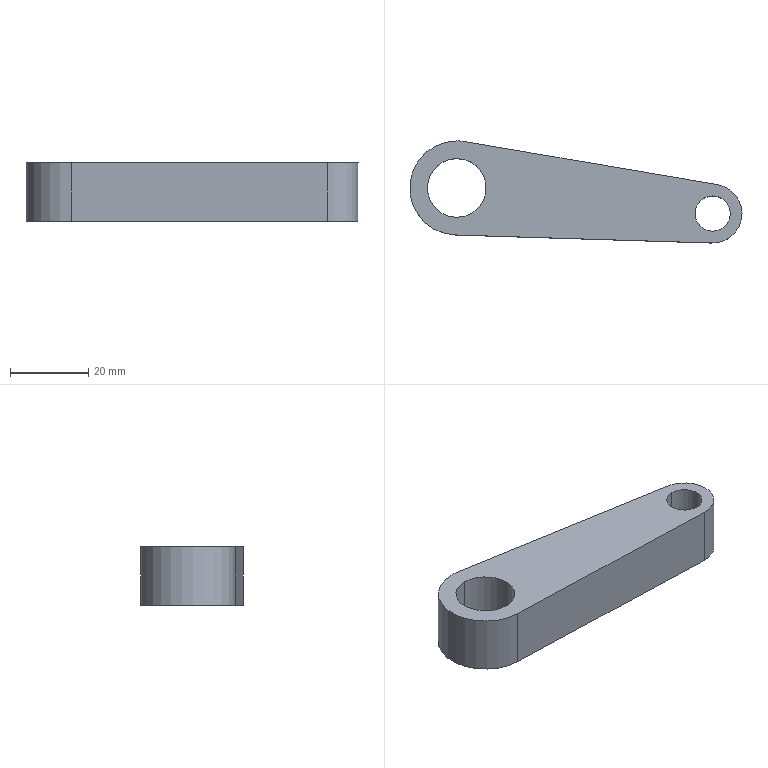Part | SolidWorks | features BaseBody 1 | 1 solid | 11 faces | box 84.765 x 26.042 x 15 mm | volume 20344 mm3 | cylinder 7 | plane 4 | commonest cylinder face diameters 15 x3 9 x2 24 x2
STEP:
#1=CARTESIAN_POINT('',(0.3749,23.994,15.));
#2=VERTEX_POINT('',#1);
#3=CARTESIAN_POINT('',(0.000000002,0.000000004,15.));
#4=VERTEX_POINT('',#3);
#5=CARTESIAN_POINT('',(0.3749,11.994,15.));
#6=DIRECTION('',(0.,0.,1.));
#7=DIRECTION('',(0.,1.,0.));
#8=AXIS2_PLACEMENT_3D('',#5,#6,#7);
#9=CIRCLE('',#8,12.);
#10=EDGE_CURVE('',#2,#4,#9,.T.);
#11=ORIENTED_EDGE('',*,*,#10,.F.);
#12=CARTESIAN_POINT('',(0.3749,23.994,0.));
#13=VERTEX_POINT('',#12);
#14=CARTESIAN_POINT('',(0.3749,23.994,15.));
#15=DIRECTION('',(0.,0.,-1.));
#16=VECTOR('',#15,1000.);
#17=LINE('',#14,#16);
#18=EDGE_CURVE('',#2,#13,#17,.T.);
#19=ORIENTED_EDGE('',*,*,#18,.T.);
#20=CARTESIAN_POINT('',(0.000000002,0.,0.));
#21=VERTEX_POINT('',#20);
#22=CARTESIAN_POINT('',(0.3749,11.994,0.));
#23=DIRECTION('',(0.,0.,-1.));
#24=DIRECTION('',(0.,1.,0.));
#25=AXIS2_PLACEMENT_3D('',#22,#23,#24);
#26=CIRCLE('',#25,12.);
#27=EDGE_CURVE('',#21,#13,#26,.T.);
#28=ORIENTED_EDGE('',*,*,#27,.F.);
#29=CARTESIAN_POINT('',(0.000000004,0.,7.5));
#30=DIRECTION('',(0.,0.,-1.));
#31=VECTOR('',#30,1000.);
#32=LINE('',#29,#31);
#33=EDGE_CURVE('',#4,#21,#32,.T.);
#34=ORIENTED_EDGE('',*,*,#33,.F.);
#35=EDGE_LOOP('',(#11,#19,#28,#34));
#36=FACE_OUTER_BOUND('',#35,.T.);
#37=CARTESIAN_POINT('',(0.3749,11.994,15.));
#38=DIRECTION('',(0.,0.,-1.));
#39=DIRECTION('',(0.,1.,0.));
#40=AXIS2_PLACEMENT_3D('',#37,#38,#39);
#41=CYLINDRICAL_SURFACE('',#40,12.);
#42=ADVANCED_FACE('',(#36),#41,.T.);
#43=CARTESIAN_POINT('',(65.64,0.9519,15.));
#44=VERTEX_POINT('',#43);
#45=CARTESIAN_POINT('',(65.64,9.952,15.));
#46=VERTEX_POINT('',#45);
#47=CARTESIAN_POINT('',(65.64,5.452,15.));
#48=DIRECTION('',(0.,0.,-1.));
#49=DIRECTION('',(0.,1.,0.));
#50=AXIS2_PLACEMENT_3D('',#47,#48,#49);
#51=CIRCLE('',#50,4.5);
#52=EDGE_CURVE('',#44,#46,#51,.T.);
#53=ORIENTED_EDGE('',*,*,#52,.F.);
#54=CARTESIAN_POINT('',(65.64,0.9519,0.));
#55=VERTEX_POINT('',#54);
#56=CARTESIAN_POINT('',(65.64,0.9519,15.));
#57=DIRECTION('',(0.,0.,-1.));
#58=VECTOR('',#57,1000.);
#59=LINE('',#56,#58);
#60=EDGE_CURVE('',#44,#55,#59,.T.);
#61=ORIENTED_EDGE('',*,*,#60,.T.);
#62=CARTESIAN_POINT('',(65.64,9.952,0.));
#63=VERTEX_POINT('',#62);
#64=CARTESIAN_POINT('',(65.64,5.452,0.));
#65=DIRECTION('',(0.,0.,-1.));
#66=DIRECTION('',(0.,1.,0.));
#67=AXIS2_PLACEMENT_3D('',#64,#65,#66);
#68=CIRCLE('',#67,4.5);
#69=EDGE_CURVE('',#55,#63,#68,.T.);
#70=ORIENTED_EDGE('',*,*,#69,.T.);
#71=CARTESIAN_POINT('',(65.64,9.952,15.));
#72=DIRECTION('',(0.,0.,-1.));
#73=VECTOR('',#72,1000.);
#74=LINE('',#71,#73);
#75=EDGE_CURVE('',#46,#63,#74,.T.);
#76=ORIENTED_EDGE('',*,*,#75,.F.);
#77=EDGE_LOOP('',(#53,#61,#70,#76));
#78=FACE_OUTER_BOUND('',#77,.T.);
#79=CARTESIAN_POINT('',(65.64,5.452,15.));
#80=DIRECTION('',(0.,0.,-1.));
#81=DIRECTION('',(0.,1.,0.));
#82=AXIS2_PLACEMENT_3D('',#79,#80,#81);
#83=CYLINDRICAL_SURFACE('',#82,4.5);
#84=ADVANCED_FACE('',(#78),#83,.F.);
#85=CARTESIAN_POINT('',(0.3749,4.494,15.));
#86=VERTEX_POINT('',#85);
#87=CARTESIAN_POINT('',(0.3749,19.494,15.));
#88=VERTEX_POINT('',#87);
#89=CARTESIAN_POINT('',(0.3749,11.994,15.));
#90=DIRECTION('',(0.,0.,-1.));
#91=DIRECTION('',(0.,1.,0.));
#92=AXIS2_PLACEMENT_3D('',#89,#90,#91);
#93=CIRCLE('',#92,7.5);
#94=EDGE_CURVE('',#86,#88,#93,.T.);
#95=ORIENTED_EDGE('',*,*,#94,.F.);
#96=CARTESIAN_POINT('',(0.3749,4.494,0.));
#97=VERTEX_POINT('',#96);
#98=CARTESIAN_POINT('',(0.3749,4.494,15.));
#99=DIRECTION('',(0.,0.,-1.));
#100=VECTOR('',#99,1000.);
#101=LINE('',#98,#100);
#102=EDGE_CURVE('',#86,#97,#101,.T.);
#103=ORIENTED_EDGE('',*,*,#102,.T.);
#104=CARTESIAN_POINT('',(0.3749,19.494,0.));
#105=VERTEX_POINT('',#104);
#106=CARTESIAN_POINT('',(0.3749,11.994,0.));
#107=DIRECTION('',(0.,0.,-1.));
#108=DIRECTION('',(0.,1.,0.));
#109=AXIS2_PLACEMENT_3D('',#106,#107,#108);
#110=CIRCLE('',#109,7.5);
#111=EDGE_CURVE('',#97,#105,#110,.T.);
#112=ORIENTED_EDGE('',*,*,#111,.T.);
#113=CARTESIAN_POINT('',(0.3749,19.494,15.));
#114=DIRECTION('',(0.,0.,-1.));
#115=VECTOR('',#114,1000.);
#116=LINE('',#113,#115);
#117=EDGE_CURVE('',#88,#105,#116,.T.);
#118=ORIENTED_EDGE('',*,*,#117,.F.);
#119=EDGE_LOOP('',(#95,#103,#112,#118));
#120=FACE_OUTER_BOUND('',#119,.T.);
#121=CARTESIAN_POINT('',(0.3749,11.994,15.));
#122=DIRECTION('',(0.,0.,-1.));
#123=DIRECTION('',(0.,1.,0.));
#124=AXIS2_PLACEMENT_3D('',#121,#122,#123);
#125=CYLINDRICAL_SURFACE('',#124,7.5);
#126=ADVANCED_FACE('',(#120),#125,.F.);
#127=ORIENTED_EDGE('',*,*,#18,.F.);
#128=CARTESIAN_POINT('',(2.388,23.824,15.));
#129=VERTEX_POINT('',#128);
#130=CARTESIAN_POINT('',(0.3749,11.994,15.));
#131=DIRECTION('',(0.,0.,1.));
#132=DIRECTION('',(0.,1.,0.));
#133=AXIS2_PLACEMENT_3D('',#130,#131,#132);
#134=CIRCLE('',#133,12.);
#135=EDGE_CURVE('',#129,#2,#134,.T.);
#136=ORIENTED_EDGE('',*,*,#135,.F.);
#137=CARTESIAN_POINT('',(2.388,23.824,0.));
#138=VERTEX_POINT('',#137);
#139=CARTESIAN_POINT('',(2.388,23.824,7.5));
#140=DIRECTION('',(0.,0.,1.));
#141=VECTOR('',#140,1000.);
#142=LINE('',#139,#141);
#143=EDGE_CURVE('',#138,#129,#142,.T.);
#144=ORIENTED_EDGE('',*,*,#143,.F.);
#145=CARTESIAN_POINT('',(0.3749,11.994,0.));
#146=DIRECTION('',(0.,0.,-1.));
#147=DIRECTION('',(0.,1.,0.));
#148=AXIS2_PLACEMENT_3D('',#145,#146,#147);
#149=CIRCLE('',#148,12.);
#150=EDGE_CURVE('',#13,#138,#149,.T.);
#151=ORIENTED_EDGE('',*,*,#150,.F.);
#152=EDGE_LOOP('',(#127,#136,#144,#151));
#153=FACE_OUTER_BOUND('',#152,.T.);
#154=CARTESIAN_POINT('',(0.3749,11.994,15.));
#155=DIRECTION('',(0.,0.,-1.));
#156=DIRECTION('',(0.,1.,0.));
#157=AXIS2_PLACEMENT_3D('',#154,#155,#156);
#158=CYLINDRICAL_SURFACE('',#157,12.);
#159=ADVANCED_FACE('',(#153),#158,.T.);
#160=CARTESIAN_POINT('',(65.64,5.452,15.));
#161=DIRECTION('',(0.,0.,-1.));
#162=DIRECTION('',(0.,1.,0.));
#163=AXIS2_PLACEMENT_3D('',#160,#161,#162);
#164=CIRCLE('',#163,4.5);
#165=EDGE_CURVE('',#46,#44,#164,.T.);
#166=ORIENTED_EDGE('',*,*,#165,.T.);
#167=ORIENTED_EDGE('',*,*,#52,.T.);
#168=EDGE_LOOP('',(#166,#167));
#169=FACE_BOUND('',#168,.T.);
#170=CARTESIAN_POINT('',(0.3749,11.994,15.));
#171=DIRECTION('',(0.,0.,-1.));
#172=DIRECTION('',(0.,1.,0.));
#173=AXIS2_PLACEMENT_3D('',#170,#171,#172);
#174=CIRCLE('',#173,7.5);
#175=EDGE_CURVE('',#88,#86,#174,.T.);
#176=ORIENTED_EDGE('',*,*,#175,.T.);
#177=ORIENTED_EDGE('',*,*,#94,.T.);
#178=EDGE_LOOP('',(#176,#177));
#179=FACE_BOUND('',#178,.T.);
#180=CARTESIAN_POINT('',(66.898,12.846,15.));
#181=VERTEX_POINT('',#180);
#182=CARTESIAN_POINT('',(66.898,12.846,15.));
#183=DIRECTION('',(-0.9858,0.1678,0.));
#184=VECTOR('',#183,1000.);
#185=LINE('',#182,#184);
#186=EDGE_CURVE('',#181,#129,#185,.T.);
#187=ORIENTED_EDGE('',*,*,#186,.T.);
#188=ORIENTED_EDGE('',*,*,#135,.T.);
#189=ORIENTED_EDGE('',*,*,#10,.T.);
#190=CARTESIAN_POINT('',(65.406,-2.044,15.));
#191=VERTEX_POINT('',#190);
#192=CARTESIAN_POINT('',(0.000000015,0.000000009,15.));
#193=DIRECTION('',(0.9995,-0.03124,0.));
#194=VECTOR('',#193,1000.);
#195=LINE('',#192,#194);
#196=EDGE_CURVE('',#4,#191,#195,.T.);
#197=ORIENTED_EDGE('',*,*,#196,.T.);
#198=CARTESIAN_POINT('',(65.64,5.452,15.));
#199=DIRECTION('',(0.,0.,1.));
#200=DIRECTION('',(0.,1.,0.));
#201=AXIS2_PLACEMENT_3D('',#198,#199,#200);
#202=CIRCLE('',#201,7.5);
#203=EDGE_CURVE('',#191,#181,#202,.T.);
#204=ORIENTED_EDGE('',*,*,#203,.T.);
#205=EDGE_LOOP('',(#187,#188,#189,#197,#204));
#206=FACE_OUTER_BOUND('',#205,.T.);
#207=CARTESIAN_POINT('',(-12.134,-2.204,15.));
#208=DIRECTION('',(0.,0.,1.));
#209=DIRECTION('',(1.,0.,0.));
#210=AXIS2_PLACEMENT_3D('',#207,#208,#209);
#211=PLANE('',#210);
#212=ADVANCED_FACE('',(#169,#179,#206),#211,.T.);
#213=CARTESIAN_POINT('',(65.64,5.452,0.));
#214=DIRECTION('',(0.,0.,-1.));
#215=DIRECTION('',(0.,1.,0.));
#216=AXIS2_PLACEMENT_3D('',#213,#214,#215);
#217=CIRCLE('',#216,4.5);
#218=EDGE_CURVE('',#63,#55,#217,.T.);
#219=ORIENTED_EDGE('',*,*,#218,.F.);
#220=ORIENTED_EDGE('',*,*,#69,.F.);
#221=EDGE_LOOP('',(#219,#220));
#222=FACE_BOUND('',#221,.T.);
#223=CARTESIAN_POINT('',(0.3749,11.994,0.));
#224=DIRECTION('',(0.,0.,-1.));
#225=DIRECTION('',(0.,1.,0.));
#226=AXIS2_PLACEMENT_3D('',#223,#224,#225);
#227=CIRCLE('',#226,7.5);
#228=EDGE_CURVE('',#105,#97,#227,.T.);
#229=ORIENTED_EDGE('',*,*,#228,.F.);
#230=ORIENTED_EDGE('',*,*,#111,.F.);
#231=EDGE_LOOP('',(#229,#230));
#232=FACE_BOUND('',#231,.T.);
#233=ORIENTED_EDGE('',*,*,#27,.T.);
#234=ORIENTED_EDGE('',*,*,#150,.T.);
#235=CARTESIAN_POINT('',(66.898,12.846,0.));
#236=VERTEX_POINT('',#235);
#237=CARTESIAN_POINT('',(2.388,23.824,0.));
#238=DIRECTION('',(-0.9858,0.1678,0.));
#239=VECTOR('',#238,1000.);
#240=LINE('',#237,#239);
#241=EDGE_CURVE('',#236,#138,#240,.T.);
#242=ORIENTED_EDGE('',*,*,#241,.F.);
#243=CARTESIAN_POINT('',(65.406,-2.044,0.));
#244=VERTEX_POINT('',#243);
#245=CARTESIAN_POINT('',(65.64,5.452,0.));
#246=DIRECTION('',(0.,0.,1.));
#247=DIRECTION('',(0.,1.,0.));
#248=AXIS2_PLACEMENT_3D('',#245,#246,#247);
#249=CIRCLE('',#248,7.5);
#250=EDGE_CURVE('',#244,#236,#249,.T.);
#251=ORIENTED_EDGE('',*,*,#250,.F.);
#252=CARTESIAN_POINT('',(65.406,-2.044,0.));
#253=DIRECTION('',(0.9995,-0.03124,0.));
#254=VECTOR('',#253,1000.);
#255=LINE('',#252,#254);
#256=EDGE_CURVE('',#21,#244,#255,.T.);
#257=ORIENTED_EDGE('',*,*,#256,.F.);
#258=EDGE_LOOP('',(#233,#234,#242,#251,#257));
#259=FACE_OUTER_BOUND('',#258,.T.);
#260=CARTESIAN_POINT('',(-12.134,-2.204,0.));
#261=DIRECTION('',(0.,0.,1.));
#262=DIRECTION('',(1.,0.,0.));
#263=AXIS2_PLACEMENT_3D('',#260,#261,#262);
#264=PLANE('',#263);
#265=ADVANCED_FACE('',(#222,#232,#259),#264,.F.);
#266=CARTESIAN_POINT('',(65.406,-2.044,7.5));
#267=DIRECTION('',(0.,0.,-1.));
#268=VECTOR('',#267,1000.);
#269=LINE('',#266,#268);
#270=EDGE_CURVE('',#191,#244,#269,.T.);
#271=ORIENTED_EDGE('',*,*,#270,.F.);
#272=ORIENTED_EDGE('',*,*,#196,.F.);
#273=ORIENTED_EDGE('',*,*,#33,.T.);
#274=ORIENTED_EDGE('',*,*,#256,.T.);
#275=EDGE_LOOP('',(#271,#272,#273,#274));
#276=FACE_OUTER_BOUND('',#275,.T.);
#277=CARTESIAN_POINT('',(65.406,-2.044,0.));
#278=DIRECTION('',(0.03124,0.9995,0.));
#279=DIRECTION('',(-0.9995,0.03124,0.));
#280=AXIS2_PLACEMENT_3D('',#277,#278,#279);
#281=PLANE('',#280);
#282=ADVANCED_FACE('',(#276),#281,.F.);
#283=ORIENTED_EDGE('',*,*,#60,.F.);
#284=ORIENTED_EDGE('',*,*,#165,.F.);
#285=ORIENTED_EDGE('',*,*,#75,.T.);
#286=ORIENTED_EDGE('',*,*,#218,.T.);
#287=EDGE_LOOP('',(#283,#284,#285,#286));
#288=FACE_OUTER_BOUND('',#287,.T.);
#289=CARTESIAN_POINT('',(65.64,5.452,15.));
#290=DIRECTION('',(0.,0.,-1.));
#291=DIRECTION('',(0.,1.,0.));
#292=AXIS2_PLACEMENT_3D('',#289,#290,#291);
#293=CYLINDRICAL_SURFACE('',#292,4.5);
#294=ADVANCED_FACE('',(#288),#293,.F.);
#295=ORIENTED_EDGE('',*,*,#102,.F.);
#296=ORIENTED_EDGE('',*,*,#175,.F.);
#297=ORIENTED_EDGE('',*,*,#117,.T.);
#298=ORIENTED_EDGE('',*,*,#228,.T.);
#299=EDGE_LOOP('',(#295,#296,#297,#298));
#300=FACE_OUTER_BOUND('',#299,.T.);
#301=CARTESIAN_POINT('',(0.3749,11.994,15.));
#302=DIRECTION('',(0.,0.,-1.));
#303=DIRECTION('',(0.,1.,0.));
#304=AXIS2_PLACEMENT_3D('',#301,#302,#303);
#305=CYLINDRICAL_SURFACE('',#304,7.5);
#306=ADVANCED_FACE('',(#300),#305,.F.);
#307=ORIENTED_EDGE('',*,*,#143,.T.);
#308=ORIENTED_EDGE('',*,*,#186,.F.);
#309=CARTESIAN_POINT('',(66.898,12.846,7.5));
#310=DIRECTION('',(0.,0.,1.));
#311=VECTOR('',#310,1000.);
#312=LINE('',#309,#311);
#313=EDGE_CURVE('',#236,#181,#312,.T.);
#314=ORIENTED_EDGE('',*,*,#313,.F.);
#315=ORIENTED_EDGE('',*,*,#241,.T.);
#316=EDGE_LOOP('',(#307,#308,#314,#315));
#317=FACE_OUTER_BOUND('',#316,.T.);
#318=CARTESIAN_POINT('',(2.388,23.824,0.));
#319=DIRECTION('',(-0.1678,-0.9858,0.));
#320=DIRECTION('',(0.9858,-0.1678,0.));
#321=AXIS2_PLACEMENT_3D('',#318,#319,#320);
#322=PLANE('',#321);
#323=ADVANCED_FACE('',(#317),#322,.F.);
#324=ORIENTED_EDGE('',*,*,#270,.T.);
#325=ORIENTED_EDGE('',*,*,#250,.T.);
#326=ORIENTED_EDGE('',*,*,#313,.T.);
#327=ORIENTED_EDGE('',*,*,#203,.F.);
#328=EDGE_LOOP('',(#324,#325,#326,#327));
#329=FACE_OUTER_BOUND('',#328,.T.);
#330=CARTESIAN_POINT('',(65.64,5.452,15.));
#331=DIRECTION('',(0.,0.,-1.));
#332=DIRECTION('',(0.,1.,0.));
#333=AXIS2_PLACEMENT_3D('',#330,#331,#332);
#334=CYLINDRICAL_SURFACE('',#333,7.5);
#335=ADVANCED_FACE('',(#329),#334,.T.);
#336=CLOSED_SHELL('',(#42,#84,#126,#159,#212,#265,#282,#294,#306,#323,#335));
#337=MANIFOLD_SOLID_BREP('',#336);
#338=CARTESIAN_POINT('',(0.,0.,0.));
#339=DIRECTION('',(0.,0.,1.));
#340=DIRECTION('',(1.,0.,0.));
#341=AXIS2_PLACEMENT_3D('',#338,#339,#340);
#342=(LENGTH_UNIT()NAMED_UNIT(*)SI_UNIT(.MILLI.,.METRE.));
#343=UNCERTAINTY_MEASURE_WITH_UNIT(LENGTH_MEASURE(0.00001),#342,'','');
#344=(NAMED_UNIT(*)PLANE_ANGLE_UNIT()SI_UNIT($,.RADIAN.));
#345=(NAMED_UNIT(*)SI_UNIT($,.STERADIAN.)SOLID_ANGLE_UNIT());
#346=(GEOMETRIC_REPRESENTATION_CONTEXT(3)GLOBAL_UNCERTAINTY_ASSIGNED_CONTEXT((#343))GLOBAL_UNIT_ASSIGNED_CONTEXT((#342,#344,#345))REPRESENTATION_CONTEXT('',''));
#347=ADVANCED_BREP_SHAPE_REPRESENTATION('',(#337,#341),#346);